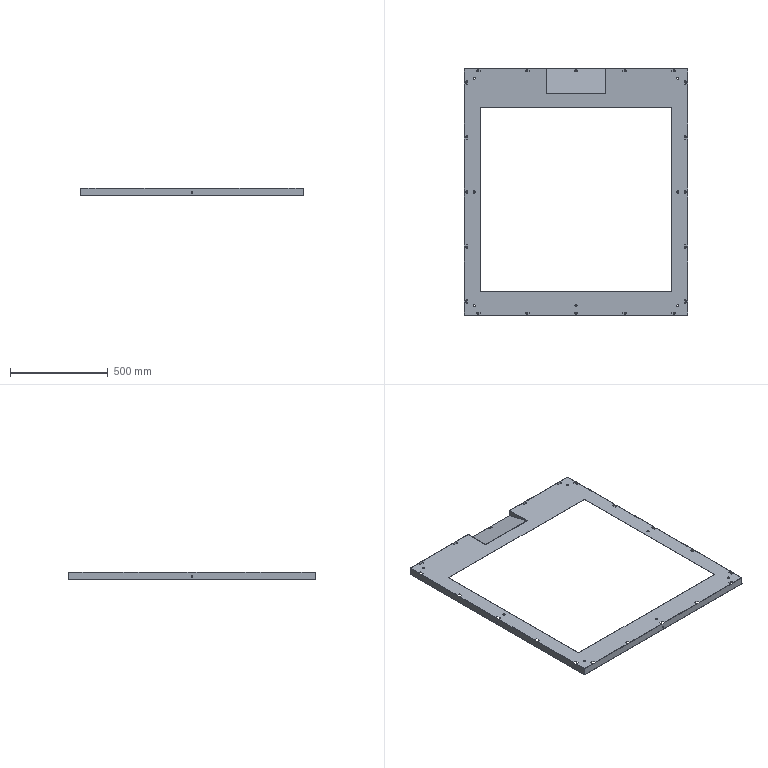Part | SolidWorks | 2 solids | 408 faces | box 1139 x 1259 x 40 mm | volume 807129 mm3 | plane 258 | cylinder 130 | spline 20 | commonest cylinder face diameters 7 x50 0.4 x30 2.4 x30 11 x14 10 x6